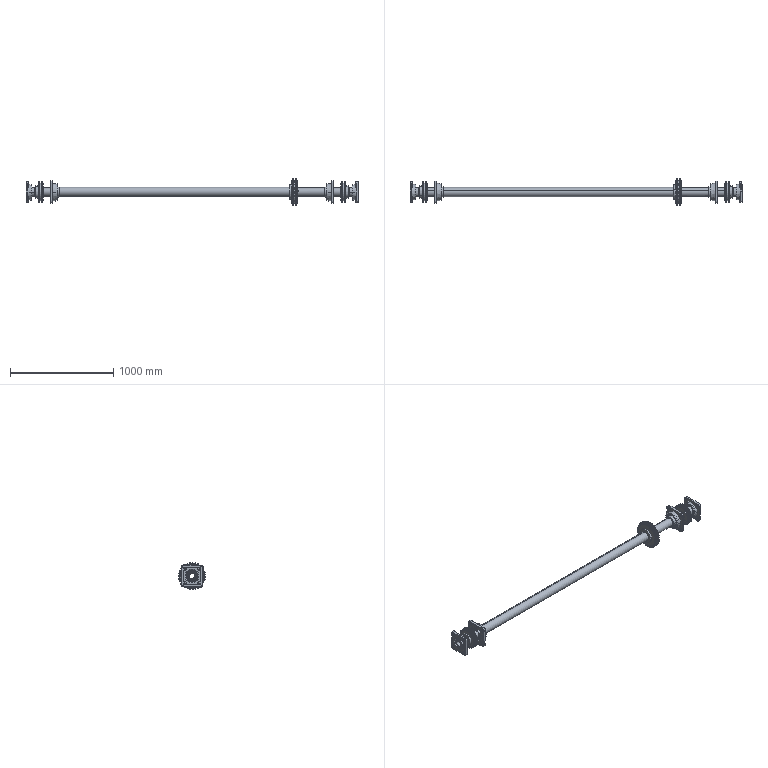Part | SolidWorks | features ReferencePattern 3, MirrorCompFeat 1 | 76 solids | 2440 faces | box 3215 x 262.517 x 262.783 mm | volume 19803434 mm3 | cylinder 1340 | plane 514 | torus 392 | sphere 152 | cone 42 | commonest cylinder face diameters 41.467 x330 16.059 x204 22.999 x200 22.826 x132 206 x96 263 x62